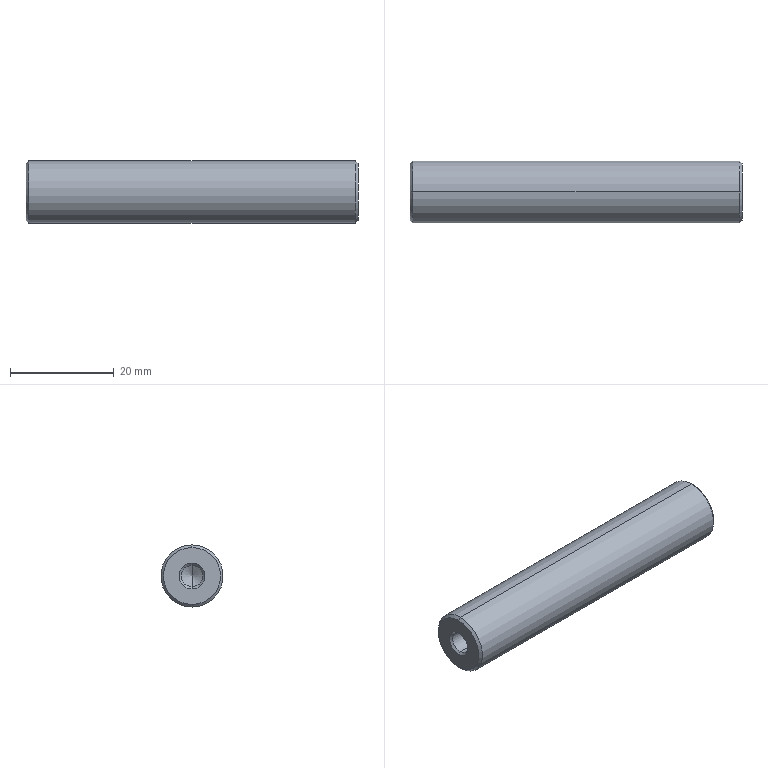Part | STEP file | PSFGT12_64_M5_PSFGT12-64-M5 | 1 solid | 14 faces | box 64 x 12 x 12 mm | volume 7075 mm3 | cone 8 | cylinder 4 | plane 2 | commonest cylinder face diameters 4.134 x2 12 x2
STEP:
#1=CARTESIAN_POINT('',(0.,0.,0.));
#2=DIRECTION('',(0.,0.,1.));
#3=DIRECTION('',(1.,0.,0.));
#4=AXIS2_PLACEMENT_3D('',#1,#2,#3);
#5=CARTESIAN_POINT('',(11.,0.,-2.067));
#6=VERTEX_POINT('',#5);
#7=CARTESIAN_POINT('',(11.,0.,2.067));
#8=VERTEX_POINT('',#7);
#9=CARTESIAN_POINT('',(11.,0.,0.));
#10=DIRECTION('',(-1.,0.,0.));
#11=DIRECTION('',(0.,0.,1.));
#12=AXIS2_PLACEMENT_3D('',#9,#10,#11);
#13=CIRCLE('',#12,2.067);
#14=CARTESIAN_POINT('',(-987.807,0.,0.));
#15=DIRECTION('',(-1.,0.,0.));
#16=DIRECTION('',(0.,0.,1.));
#17=AXIS2_PLACEMENT_3D('',#14,#15,#16);
#18=CONICAL_SURFACE('',#17,1732.051,1.047);
#19=CARTESIAN_POINT('',(0.,-998.807));
#20=DIRECTION('',(1.,0.));
#21=VECTOR('',#20,1.);
#22=LINE('',#19,#21);
#23=(GEOMETRIC_REPRESENTATION_CONTEXT(2)PARAMETRIC_REPRESENTATION_CONTEXT()REPRESENTATION_CONTEXT('',''));
#24=DEFINITIONAL_REPRESENTATION('',(#22),#23);
#25=PCURVE('',#18,#24);
#26=CARTESIAN_POINT('',(12.193,0.,0.));
#27=DIRECTION('',(-1.,0.,0.));
#28=DIRECTION('',(0.,0.,1.));
#29=AXIS2_PLACEMENT_3D('',#26,#27,#28);
#30=CYLINDRICAL_SURFACE('',#29,2.067);
#31=CARTESIAN_POINT('',(0.,1.193));
#32=DIRECTION('',(1.,0.));
#33=VECTOR('',#32,1.);
#34=LINE('',#31,#33);
#35=(GEOMETRIC_REPRESENTATION_CONTEXT(2)PARAMETRIC_REPRESENTATION_CONTEXT()REPRESENTATION_CONTEXT('',''));
#36=DEFINITIONAL_REPRESENTATION('',(#34),#35);
#37=PCURVE('',#30,#36);
#38=SURFACE_CURVE('',#13,(#25,#37),.PCURVE_S1.);
#39=EDGE_CURVE('',#6,#8,#38,.T.);
#40=ORIENTED_EDGE('',*,*,#39,.F.);
#41=CARTESIAN_POINT('',(12.193,0.,0.));
#42=VERTEX_POINT('',#41);
#43=CARTESIAN_POINT('',(12.193,0.,0.));
#44=DIRECTION('',(-0.5,0.,-0.866));
#45=VECTOR('',#44,1.);
#46=LINE('',#43,#45);
#47=CARTESIAN_POINT('',(3.142,-1000.));
#48=CARTESIAN_POINT('',(3.142,-999.982));
#49=CARTESIAN_POINT('',(3.142,-999.946));
#50=CARTESIAN_POINT('',(3.142,-999.892));
#51=CARTESIAN_POINT('',(3.142,-999.837));
#52=CARTESIAN_POINT('',(3.142,-999.783));
#53=CARTESIAN_POINT('',(3.142,-999.729));
#54=CARTESIAN_POINT('',(3.142,-999.675));
#55=CARTESIAN_POINT('',(3.142,-999.62));
#56=CARTESIAN_POINT('',(3.142,-999.566));
#57=CARTESIAN_POINT('',(3.142,-999.512));
#58=CARTESIAN_POINT('',(3.142,-999.458));
#59=CARTESIAN_POINT('',(3.142,-999.403));
#60=CARTESIAN_POINT('',(3.142,-999.349));
#61=CARTESIAN_POINT('',(3.142,-999.295));
#62=CARTESIAN_POINT('',(3.142,-999.241));
#63=CARTESIAN_POINT('',(3.142,-999.186));
#64=CARTESIAN_POINT('',(3.142,-999.132));
#65=CARTESIAN_POINT('',(3.142,-999.078));
#66=CARTESIAN_POINT('',(3.142,-999.024));
#67=CARTESIAN_POINT('',(3.142,-998.969));
#68=CARTESIAN_POINT('',(3.142,-998.915));
#69=CARTESIAN_POINT('',(3.142,-998.861));
#70=CARTESIAN_POINT('',(3.142,-998.825));
#71=CARTESIAN_POINT('',(3.142,-998.807));
#72=B_SPLINE_CURVE_WITH_KNOTS('',3,(#47,#48,#49,#50,#51,#52,#53,#54,#55,#56,#57,#58,#59,#60,#61,#62,#63,#64,#65,#66,#67,#68,#69,#70,#71),.UNSPECIFIED.,.F.,.F.,(4,1,1,1,1,1,1,1,1,1,1,1,1,1,1,1,1,1,1,1,1,1,4),(0.,0.1085,0.217,0.3255,0.434,0.5424,0.6509,0.7594,0.8679,0.9764,1.085,1.193,1.302,1.41,1.519,1.627,1.736,1.844,1.953,2.061,2.17,2.278,2.387),.QUASI_UNIFORM_KNOTS.);
#73=(GEOMETRIC_REPRESENTATION_CONTEXT(2)PARAMETRIC_REPRESENTATION_CONTEXT()REPRESENTATION_CONTEXT('',''));
#74=DEFINITIONAL_REPRESENTATION('',(#72),#73);
#75=PCURVE('',#18,#74);
#76=CARTESIAN_POINT('',(-987.807,0.,0.));
#77=DIRECTION('',(-1.,0.,0.));
#78=DIRECTION('',(0.,0.,1.));
#79=AXIS2_PLACEMENT_3D('',#76,#77,#78);
#80=CONICAL_SURFACE('',#79,1732.051,1.047);
#81=CARTESIAN_POINT('',(3.142,-1000.));
#82=CARTESIAN_POINT('',(3.142,-999.982));
#83=CARTESIAN_POINT('',(3.142,-999.946));
#84=CARTESIAN_POINT('',(3.142,-999.892));
#85=CARTESIAN_POINT('',(3.142,-999.837));
#86=CARTESIAN_POINT('',(3.142,-999.783));
#87=CARTESIAN_POINT('',(3.142,-999.729));
#88=CARTESIAN_POINT('',(3.142,-999.675));
#89=CARTESIAN_POINT('',(3.142,-999.62));
#90=CARTESIAN_POINT('',(3.142,-999.566));
#91=CARTESIAN_POINT('',(3.142,-999.512));
#92=CARTESIAN_POINT('',(3.142,-999.458));
#93=CARTESIAN_POINT('',(3.142,-999.403));
#94=CARTESIAN_POINT('',(3.142,-999.349));
#95=CARTESIAN_POINT('',(3.142,-999.295));
#96=CARTESIAN_POINT('',(3.142,-999.241));
#97=CARTESIAN_POINT('',(3.142,-999.186));
#98=CARTESIAN_POINT('',(3.142,-999.132));
#99=CARTESIAN_POINT('',(3.142,-999.078));
#100=CARTESIAN_POINT('',(3.142,-999.024));
#101=CARTESIAN_POINT('',(3.142,-998.969));
#102=CARTESIAN_POINT('',(3.142,-998.915));
#103=CARTESIAN_POINT('',(3.142,-998.861));
#104=CARTESIAN_POINT('',(3.142,-998.825));
#105=CARTESIAN_POINT('',(3.142,-998.807));
#106=B_SPLINE_CURVE_WITH_KNOTS('',3,(#81,#82,#83,#84,#85,#86,#87,#88,#89,#90,#91,#92,#93,#94,#95,#96,#97,#98,#99,#100,#101,#102,#103,#104,#105),.UNSPECIFIED.,.F.,.F.,(4,1,1,1,1,1,1,1,1,1,1,1,1,1,1,1,1,1,1,1,1,1,4),(0.,0.1085,0.217,0.3255,0.434,0.5424,0.6509,0.7594,0.8679,0.9764,1.085,1.193,1.302,1.41,1.519,1.627,1.736,1.844,1.953,2.061,2.17,2.278,2.387),.QUASI_UNIFORM_KNOTS.);
#107=(GEOMETRIC_REPRESENTATION_CONTEXT(2)PARAMETRIC_REPRESENTATION_CONTEXT()REPRESENTATION_CONTEXT('',''));
#108=DEFINITIONAL_REPRESENTATION('',(#106),#107);
#109=PCURVE('',#80,#108);
#110=SURFACE_CURVE('',#46,(#75,#109),.PCURVE_S1.);
#111=EDGE_CURVE('',#42,#6,#110,.T.);
#112=ORIENTED_EDGE('',*,*,#111,.F.);
#113=CARTESIAN_POINT('',(12.193,0.,0.));
#114=DIRECTION('',(-0.5,0.,0.866));
#115=VECTOR('',#114,1.);
#116=LINE('',#113,#115);
#117=CARTESIAN_POINT('',(6.283,-1000.));
#118=DIRECTION('',(0.,1.));
#119=VECTOR('',#118,1.);
#120=LINE('',#117,#119);
#121=(GEOMETRIC_REPRESENTATION_CONTEXT(2)PARAMETRIC_REPRESENTATION_CONTEXT()REPRESENTATION_CONTEXT('',''));
#122=DEFINITIONAL_REPRESENTATION('',(#120),#121);
#123=PCURVE('',#18,#122);
#124=CARTESIAN_POINT('',(0.,-1000.));
#125=DIRECTION('',(0.,1.));
#126=VECTOR('',#125,1.);
#127=LINE('',#124,#126);
#128=(GEOMETRIC_REPRESENTATION_CONTEXT(2)PARAMETRIC_REPRESENTATION_CONTEXT()REPRESENTATION_CONTEXT('',''));
#129=DEFINITIONAL_REPRESENTATION('',(#127),#128);
#130=PCURVE('',#80,#129);
#131=SURFACE_CURVE('',#116,(#123,#130),.PCURVE_S1.);
#132=EDGE_CURVE('',#42,#8,#131,.T.);
#133=ORIENTED_EDGE('',*,*,#132,.T.);
#134=EDGE_LOOP('',(#40,#112,#133));
#135=FACE_BOUND('',#134,.F.);
#136=ADVANCED_FACE('',(#135),#18,.F.);
#137=CARTESIAN_POINT('',(0.433,0.,2.067));
#138=VERTEX_POINT('',#137);
#139=CARTESIAN_POINT('',(12.193,0.,2.067));
#140=DIRECTION('',(-1.,0.,0.));
#141=VECTOR('',#140,1.);
#142=LINE('',#139,#141);
#143=CARTESIAN_POINT('',(6.283,0.));
#144=DIRECTION('',(0.,1.));
#145=VECTOR('',#144,1.);
#146=LINE('',#143,#145);
#147=(GEOMETRIC_REPRESENTATION_CONTEXT(2)PARAMETRIC_REPRESENTATION_CONTEXT()REPRESENTATION_CONTEXT('',''));
#148=DEFINITIONAL_REPRESENTATION('',(#146),#147);
#149=PCURVE('',#30,#148);
#150=CARTESIAN_POINT('',(12.193,0.,0.));
#151=DIRECTION('',(-1.,0.,0.));
#152=DIRECTION('',(0.,0.,1.));
#153=AXIS2_PLACEMENT_3D('',#150,#151,#152);
#154=CYLINDRICAL_SURFACE('',#153,2.067);
#155=CARTESIAN_POINT('',(0.,0.));
#156=DIRECTION('',(0.,1.));
#157=VECTOR('',#156,1.);
#158=LINE('',#155,#157);
#159=(GEOMETRIC_REPRESENTATION_CONTEXT(2)PARAMETRIC_REPRESENTATION_CONTEXT()REPRESENTATION_CONTEXT('',''));
#160=DEFINITIONAL_REPRESENTATION('',(#158),#159);
#161=PCURVE('',#154,#160);
#162=SURFACE_CURVE('',#142,(#149,#161),.PCURVE_S1.);
#163=EDGE_CURVE('',#8,#138,#162,.T.);
#164=ORIENTED_EDGE('',*,*,#163,.T.);
#165=CARTESIAN_POINT('',(0.433,0.,-2.067));
#166=VERTEX_POINT('',#165);
#167=CARTESIAN_POINT('',(0.433,0.,0.));
#168=DIRECTION('',(-1.,0.,0.));
#169=DIRECTION('',(0.,0.,1.));
#170=AXIS2_PLACEMENT_3D('',#167,#168,#169);
#171=CIRCLE('',#170,2.067);
#172=CARTESIAN_POINT('',(0.,11.76));
#173=DIRECTION('',(1.,0.));
#174=VECTOR('',#173,1.);
#175=LINE('',#172,#174);
#176=(GEOMETRIC_REPRESENTATION_CONTEXT(2)PARAMETRIC_REPRESENTATION_CONTEXT()REPRESENTATION_CONTEXT('',''));
#177=DEFINITIONAL_REPRESENTATION('',(#175),#176);
#178=PCURVE('',#30,#177);
#179=CARTESIAN_POINT('',(0.433,0.,0.));
#180=DIRECTION('',(-1.,0.,0.));
#181=DIRECTION('',(0.,0.,1.));
#182=AXIS2_PLACEMENT_3D('',#179,#180,#181);
#183=CONICAL_SURFACE('',#182,2.067,0.7854);
#184=CARTESIAN_POINT('',(0.,0.));
#185=DIRECTION('',(1.,0.));
#186=VECTOR('',#185,1.);
#187=LINE('',#184,#186);
#188=(GEOMETRIC_REPRESENTATION_CONTEXT(2)PARAMETRIC_REPRESENTATION_CONTEXT()REPRESENTATION_CONTEXT('',''));
#189=DEFINITIONAL_REPRESENTATION('',(#187),#188);
#190=PCURVE('',#183,#189);
#191=SURFACE_CURVE('',#171,(#178,#190),.PCURVE_S1.);
#192=EDGE_CURVE('',#166,#138,#191,.T.);
#193=ORIENTED_EDGE('',*,*,#192,.F.);
#194=CARTESIAN_POINT('',(12.193,0.,-2.067));
#195=DIRECTION('',(-1.,0.,0.));
#196=VECTOR('',#195,1.);
#197=LINE('',#194,#196);
#198=CARTESIAN_POINT('',(3.142,0.));
#199=DIRECTION('',(0.,1.));
#200=VECTOR('',#199,1.);
#201=LINE('',#198,#200);
#202=(GEOMETRIC_REPRESENTATION_CONTEXT(2)PARAMETRIC_REPRESENTATION_CONTEXT()REPRESENTATION_CONTEXT('',''));
#203=DEFINITIONAL_REPRESENTATION('',(#201),#202);
#204=PCURVE('',#30,#203);
#205=CARTESIAN_POINT('',(3.142,0.));
#206=DIRECTION('',(0.,1.));
#207=VECTOR('',#206,1.);
#208=LINE('',#205,#207);
#209=(GEOMETRIC_REPRESENTATION_CONTEXT(2)PARAMETRIC_REPRESENTATION_CONTEXT()REPRESENTATION_CONTEXT('',''));
#210=DEFINITIONAL_REPRESENTATION('',(#208),#209);
#211=PCURVE('',#154,#210);
#212=SURFACE_CURVE('',#197,(#204,#211),.PCURVE_S1.);
#213=EDGE_CURVE('',#6,#166,#212,.T.);
#214=ORIENTED_EDGE('',*,*,#213,.F.);
#215=ORIENTED_EDGE('',*,*,#39,.T.);
#216=EDGE_LOOP('',(#164,#193,#214,#215));
#217=FACE_BOUND('',#216,.F.);
#218=ADVANCED_FACE('',(#217),#30,.F.);
#219=CARTESIAN_POINT('',(0.,0.,2.5));
#220=VERTEX_POINT('',#219);
#221=CARTESIAN_POINT('',(0.433,0.,2.067));
#222=DIRECTION('',(-0.7071,0.,0.7071));
#223=VECTOR('',#222,1.);
#224=LINE('',#221,#223);
#225=CARTESIAN_POINT('',(6.283,0.));
#226=DIRECTION('',(0.,1.));
#227=VECTOR('',#226,1.);
#228=LINE('',#225,#227);
#229=(GEOMETRIC_REPRESENTATION_CONTEXT(2)PARAMETRIC_REPRESENTATION_CONTEXT()REPRESENTATION_CONTEXT('',''));
#230=DEFINITIONAL_REPRESENTATION('',(#228),#229);
#231=PCURVE('',#183,#230);
#232=CARTESIAN_POINT('',(0.433,0.,0.));
#233=DIRECTION('',(-1.,0.,0.));
#234=DIRECTION('',(0.,0.,1.));
#235=AXIS2_PLACEMENT_3D('',#232,#233,#234);
#236=CONICAL_SURFACE('',#235,2.067,0.7854);
#237=CARTESIAN_POINT('',(0.,0.));
#238=DIRECTION('',(0.,1.));
#239=VECTOR('',#238,1.);
#240=LINE('',#237,#239);
#241=(GEOMETRIC_REPRESENTATION_CONTEXT(2)PARAMETRIC_REPRESENTATION_CONTEXT()REPRESENTATION_CONTEXT('',''));
#242=DEFINITIONAL_REPRESENTATION('',(#240),#241);
#243=PCURVE('',#236,#242);
#244=SURFACE_CURVE('',#224,(#231,#243),.PCURVE_S1.);
#245=EDGE_CURVE('',#138,#220,#244,.T.);
#246=ORIENTED_EDGE('',*,*,#245,.T.);
#247=CARTESIAN_POINT('',(0.,0.,-2.5));
#248=VERTEX_POINT('',#247);
#249=CARTESIAN_POINT('',(0.,0.,0.));
#250=DIRECTION('',(-1.,0.,0.));
#251=DIRECTION('',(0.,0.,1.));
#252=AXIS2_PLACEMENT_3D('',#249,#250,#251);
#253=CIRCLE('',#252,2.5);
#254=CARTESIAN_POINT('',(0.,0.433));
#255=DIRECTION('',(1.,0.));
#256=VECTOR('',#255,1.);
#257=LINE('',#254,#256);
#258=(GEOMETRIC_REPRESENTATION_CONTEXT(2)PARAMETRIC_REPRESENTATION_CONTEXT()REPRESENTATION_CONTEXT('',''));
#259=DEFINITIONAL_REPRESENTATION('',(#257),#258);
#260=PCURVE('',#183,#259);
#261=CARTESIAN_POINT('',(0.,0.,0.));
#262=DIRECTION('',(1.,0.,0.));
#263=DIRECTION('',(0.,0.,-1.));
#264=AXIS2_PLACEMENT_3D('',#261,#262,#263);
#265=PLANE('',#264);
#266=CARTESIAN_POINT('',(-2.5,0.));
#267=CARTESIAN_POINT('',(-2.5,4.33));
#268=CARTESIAN_POINT('',(1.25,2.165));
#269=CARTESIAN_POINT('',(5.,0.));
#270=CARTESIAN_POINT('',(1.25,-2.165));
#271=CARTESIAN_POINT('',(-2.5,-4.33));
#272=CARTESIAN_POINT('',(-2.5,0.));
#273=(BOUNDED_CURVE()B_SPLINE_CURVE(2,(#266,#267,#268,#269,#270,#271,#272),.UNSPECIFIED.,.T.,.F.)B_SPLINE_CURVE_WITH_KNOTS((1,2,2,2,2,1),(-2.094,0.,2.094,4.189,6.283,8.378),.UNSPECIFIED.)CURVE()GEOMETRIC_REPRESENTATION_ITEM()RATIONAL_B_SPLINE_CURVE((1.,0.5,1.,0.5,1.,0.5,1.))REPRESENTATION_ITEM(''));
#274=(GEOMETRIC_REPRESENTATION_CONTEXT(2)PARAMETRIC_REPRESENTATION_CONTEXT()REPRESENTATION_CONTEXT('',''));
#275=DEFINITIONAL_REPRESENTATION('',(#273),#274);
#276=PCURVE('',#265,#275);
#277=SURFACE_CURVE('',#253,(#260,#276),.PCURVE_S1.);
#278=EDGE_CURVE('',#248,#220,#277,.T.);
#279=ORIENTED_EDGE('',*,*,#278,.F.);
#280=CARTESIAN_POINT('',(0.433,0.,-2.067));
#281=DIRECTION('',(-0.7071,0.,-0.7071));
#282=VECTOR('',#281,1.);
#283=LINE('',#280,#282);
#284=CARTESIAN_POINT('',(3.142,0.));
#285=DIRECTION('',(0.,1.));
#286=VECTOR('',#285,1.);
#287=LINE('',#284,#286);
#288=(GEOMETRIC_REPRESENTATION_CONTEXT(2)PARAMETRIC_REPRESENTATION_CONTEXT()REPRESENTATION_CONTEXT('',''));
#289=DEFINITIONAL_REPRESENTATION('',(#287),#288);
#290=PCURVE('',#183,#289);
#291=CARTESIAN_POINT('',(3.142,0.));
#292=DIRECTION('',(0.,1.));
#293=VECTOR('',#292,1.);
#294=LINE('',#291,#293);
#295=(GEOMETRIC_REPRESENTATION_CONTEXT(2)PARAMETRIC_REPRESENTATION_CONTEXT()REPRESENTATION_CONTEXT('',''));
#296=DEFINITIONAL_REPRESENTATION('',(#294),#295);
#297=PCURVE('',#236,#296);
#298=SURFACE_CURVE('',#283,(#290,#297),.PCURVE_S1.);
#299=EDGE_CURVE('',#166,#248,#298,.T.);
#300=ORIENTED_EDGE('',*,*,#299,.F.);
#301=ORIENTED_EDGE('',*,*,#192,.T.);
#302=EDGE_LOOP('',(#246,#279,#300,#301));
#303=FACE_BOUND('',#302,.F.);
#304=ADVANCED_FACE('',(#303),#183,.F.);
#305=CARTESIAN_POINT('',(64.,0.,5.5));
#306=VERTEX_POINT('',#305);
#307=CARTESIAN_POINT('',(64.,0.,-5.5));
#308=VERTEX_POINT('',#307);
#309=CARTESIAN_POINT('',(64.,0.,0.));
#310=DIRECTION('',(-1.,0.,0.));
#311=DIRECTION('',(0.,0.,1.));
#312=AXIS2_PLACEMENT_3D('',#309,#310,#311);
#313=CIRCLE('',#312,5.5);
#314=CARTESIAN_POINT('',(64.,0.,0.));
#315=DIRECTION('',(-1.,0.,0.));
#316=DIRECTION('',(0.,0.,1.));
#317=AXIS2_PLACEMENT_3D('',#314,#315,#316);
#318=CONICAL_SURFACE('',#317,5.5,0.7854);
#319=CARTESIAN_POINT('',(0.,0.));
#320=DIRECTION('',(1.,0.));
#321=VECTOR('',#320,1.);
#322=LINE('',#319,#321);
#323=(GEOMETRIC_REPRESENTATION_CONTEXT(2)PARAMETRIC_REPRESENTATION_CONTEXT()REPRESENTATION_CONTEXT('',''));
#324=DEFINITIONAL_REPRESENTATION('',(#322),#323);
#325=PCURVE('',#318,#324);
#326=CARTESIAN_POINT('',(64.,5.5,0.));
#327=DIRECTION('',(-1.,0.,0.));
#328=DIRECTION('',(0.,0.,1.));
#329=AXIS2_PLACEMENT_3D('',#326,#327,#328);
#330=PLANE('',#329);
#331=CARTESIAN_POINT('',(0.,-5.5));
#332=DIRECTION('',(1.,0.));
#333=AXIS2_PLACEMENT_2D('',#331,#332);
#334=CIRCLE('',#333,5.5);
#335=(GEOMETRIC_REPRESENTATION_CONTEXT(2)PARAMETRIC_REPRESENTATION_CONTEXT()REPRESENTATION_CONTEXT('',''));
#336=DEFINITIONAL_REPRESENTATION('',(#334),#335);
#337=PCURVE('',#330,#336);
#338=SURFACE_CURVE('',#313,(#325,#337),.PCURVE_S1.);
#339=EDGE_CURVE('',#306,#308,#338,.T.);
#340=ORIENTED_EDGE('',*,*,#339,.T.);
#341=CARTESIAN_POINT('',(63.5,0.,-6.));
#342=VERTEX_POINT('',#341);
#343=CARTESIAN_POINT('',(64.,0.,-5.5));
#344=DIRECTION('',(-0.7071,0.,-0.7071));
#345=VECTOR('',#344,1.);
#346=LINE('',#343,#345);
#347=CARTESIAN_POINT('',(3.142,0.));
#348=DIRECTION('',(0.,1.));
#349=VECTOR('',#348,1.);
#350=LINE('',#347,#349);
#351=(GEOMETRIC_REPRESENTATION_CONTEXT(2)PARAMETRIC_REPRESENTATION_CONTEXT()REPRESENTATION_CONTEXT('',''));
#352=DEFINITIONAL_REPRESENTATION('',(#350),#351);
#353=PCURVE('',#318,#352);
#354=CARTESIAN_POINT('',(64.,0.,0.));
#355=DIRECTION('',(-1.,0.,0.));
#356=DIRECTION('',(0.,0.,1.));
#357=AXIS2_PLACEMENT_3D('',#354,#355,#356);
#358=CONICAL_SURFACE('',#357,5.5,0.7854);
#359=CARTESIAN_POINT('',(3.142,0.));
#360=DIRECTION('',(0.,1.));
#361=VECTOR('',#360,1.);
#362=LINE('',#359,#361);
#363=(GEOMETRIC_REPRESENTATION_CONTEXT(2)PARAMETRIC_REPRESENTATION_CONTEXT()REPRESENTATION_CONTEXT('',''));
#364=DEFINITIONAL_REPRESENTATION('',(#362),#363);
#365=PCURVE('',#358,#364);
#366=SURFACE_CURVE('',#346,(#353,#365),.PCURVE_S1.);
#367=EDGE_CURVE('',#308,#342,#366,.T.);
#368=ORIENTED_EDGE('',*,*,#367,.T.);
#369=CARTESIAN_POINT('',(63.5,0.,6.));
#370=VERTEX_POINT('',#369);
#371=CARTESIAN_POINT('',(63.5,0.,0.));
#372=DIRECTION('',(-1.,0.,0.));
#373=DIRECTION('',(0.,0.,1.));
#374=AXIS2_PLACEMENT_3D('',#371,#372,#373);
#375=CIRCLE('',#374,6.);
#376=CARTESIAN_POINT('',(0.,0.5));
#377=DIRECTION('',(1.,0.));
#378=VECTOR('',#377,1.);
#379=LINE('',#376,#378);
#380=(GEOMETRIC_REPRESENTATION_CONTEXT(2)PARAMETRIC_REPRESENTATION_CONTEXT()REPRESENTATION_CONTEXT('',''));
#381=DEFINITIONAL_REPRESENTATION('',(#379),#380);
#382=PCURVE('',#318,#381);
#383=CARTESIAN_POINT('',(64.,0.,0.));
#384=DIRECTION('',(-1.,0.,0.));
#385=DIRECTION('',(0.,0.,1.));
#386=AXIS2_PLACEMENT_3D('',#383,#384,#385);
#387=CYLINDRICAL_SURFACE('',#386,6.);
#388=CARTESIAN_POINT('',(0.,0.5));
#389=DIRECTION('',(1.,0.));
#390=VECTOR('',#389,1.);
#391=LINE('',#388,#390);
#392=(GEOMETRIC_REPRESENTATION_CONTEXT(2)PARAMETRIC_REPRESENTATION_CONTEXT()REPRESENTATION_CONTEXT('',''));
#393=DEFINITIONAL_REPRESENTATION('',(#391),#392);
#394=PCURVE('',#387,#393);
#395=SURFACE_CURVE('',#375,(#382,#394),.PCURVE_S1.);
#396=EDGE_CURVE('',#370,#342,#395,.T.);
#397=ORIENTED_EDGE('',*,*,#396,.F.);
#398=CARTESIAN_POINT('',(64.,0.,5.5));
#399=DIRECTION('',(-0.7071,0.,0.7071));
#400=VECTOR('',#399,1.);
#401=LINE('',#398,#400);
#402=CARTESIAN_POINT('',(0.,0.));
#403=DIRECTION('',(0.,1.));
#404=VECTOR('',#403,1.);
#405=LINE('',#402,#404);
#406=(GEOMETRIC_REPRESENTATION_CONTEXT(2)PARAMETRIC_REPRESENTATION_CONTEXT()REPRESENTATION_CONTEXT('',''));
#407=DEFINITIONAL_REPRESENTATION('',(#405),#406);
#408=PCURVE('',#318,#407);
#409=CARTESIAN_POINT('',(6.283,0.));
#410=DIRECTION('',(0.,1.));
#411=VECTOR('',#410,1.);
#412=LINE('',#409,#411);
#413=(GEOMETRIC_REPRESENTATION_CONTEXT(2)PARAMETRIC_REPRESENTATION_CONTEXT()REPRESENTATION_CONTEXT('',''));
#414=DEFINITIONAL_REPRESENTATION('',(#412),#413);
#415=PCURVE('',#358,#414);
#416=SURFACE_CURVE('',#401,(#408,#415),.PCURVE_S1.);
#417=EDGE_CURVE('',#306,#370,#416,.T.);
#418=ORIENTED_EDGE('',*,*,#417,.F.);
#419=EDGE_LOOP('',(#340,#368,#397,#418));
#420=FACE_BOUND('',#419,.T.);
#421=ADVANCED_FACE('',(#420),#318,.T.);
#422=ORIENTED_EDGE('',*,*,#396,.T.);
#423=CARTESIAN_POINT('',(0.5,0.,-6.));
#424=VERTEX_POINT('',#423);
#425=CARTESIAN_POINT('',(64.,0.,-6.));
#426=DIRECTION('',(-1.,0.,0.));
#427=VECTOR('',#426,1.);
#428=LINE('',#425,#427);
#429=CARTESIAN_POINT('',(3.142,0.));
#430=DIRECTION('',(0.,1.));
#431=VECTOR('',#430,1.);
#432=LINE('',#429,#431);
#433=(GEOMETRIC_REPRESENTATION_CONTEXT(2)PARAMETRIC_REPRESENTATION_CONTEXT()REPRESENTATION_CONTEXT('',''));
#434=DEFINITIONAL_REPRESENTATION('',(#432),#433);
#435=PCURVE('',#387,#434);
#436=CARTESIAN_POINT('',(64.,0.,0.));
#437=DIRECTION('',(-1.,0.,0.));
#438=DIRECTION('',(0.,0.,1.));
#439=AXIS2_PLACEMENT_3D('',#436,#437,#438);
#440=CYLINDRICAL_SURFACE('',#439,6.);
#441=CARTESIAN_POINT('',(3.142,0.));
#442=DIRECTION('',(0.,1.));
#443=VECTOR('',#442,1.);
#444=LINE('',#441,#443);
#445=(GEOMETRIC_REPRESENTATION_CONTEXT(2)PARAMETRIC_REPRESENTATION_CONTEXT()REPRESENTATION_CONTEXT('',''));
#446=DEFINITIONAL_REPRESENTATION('',(#444),#445);
#447=PCURVE('',#440,#446);
#448=SURFACE_CURVE('',#428,(#435,#447),.PCURVE_S1.);
#449=EDGE_CURVE('',#342,#424,#448,.T.);
#450=ORIENTED_EDGE('',*,*,#449,.T.);
#451=CARTESIAN_POINT('',(0.5,0.,6.));
#452=VERTEX_POINT('',#451);
#453=CARTESIAN_POINT('',(0.5,0.,0.));
#454=DIRECTION('',(-1.,0.,0.));
#455=DIRECTION('',(0.,0.,1.));
#456=AXIS2_PLACEMENT_3D('',#453,#454,#455);
#457=CIRCLE('',#456,6.);
#458=CARTESIAN_POINT('',(0.,63.5));
#459=DIRECTION('',(1.,0.));
#460=VECTOR('',#459,1.);
#461=LINE('',#458,#460);
#462=(GEOMETRIC_REPRESENTATION_CONTEXT(2)PARAMETRIC_REPRESENTATION_CONTEXT()REPRESENTATION_CONTEXT('',''));
#463=DEFINITIONAL_REPRESENTATION('',(#461),#462);
#464=PCURVE('',#387,#463);
#465=CARTESIAN_POINT('',(0.5,0.,0.));
#466=DIRECTION('',(1.,0.,0.));
#467=DIRECTION('',(0.,0.,-1.));
#468=AXIS2_PLACEMENT_3D('',#465,#466,#467);
#469=CONICAL_SURFACE('',#468,6.,0.7854);
#470=CARTESIAN_POINT('',(3.142,0.));
#471=DIRECTION('',(-1.,0.));
#472=VECTOR('',#471,1.);
#473=LINE('',#470,#472);
#474=(GEOMETRIC_REPRESENTATION_CONTEXT(2)PARAMETRIC_REPRESENTATION_CONTEXT()REPRESENTATION_CONTEXT('',''));
#475=DEFINITIONAL_REPRESENTATION('',(#473),#474);
#476=PCURVE('',#469,#475);
#477=SURFACE_CURVE('',#457,(#464,#476),.PCURVE_S1.);
#478=EDGE_CURVE('',#452,#424,#477,.T.);
#479=ORIENTED_EDGE('',*,*,#478,.F.);
#480=CARTESIAN_POINT('',(64.,0.,6.));
#481=DIRECTION('',(-1.,0.,0.));
#482=VECTOR('',#481,1.);
#483=LINE('',#480,#482);
#484=CARTESIAN_POINT('',(0.,0.));
#485=DIRECTION('',(0.,1.));
#486=VECTOR('',#485,1.);
#487=LINE('',#484,#486);
#488=(GEOMETRIC_REPRESENTATION_CONTEXT(2)PARAMETRIC_REPRESENTATION_CONTEXT()REPRESENTATION_CONTEXT('',''));
#489=DEFINITIONAL_REPRESENTATION('',(#487),#488);
#490=PCURVE('',#387,#489);
#491=CARTESIAN_POINT('',(6.283,0.));
#492=DIRECTION('',(0.,1.));
#493=VECTOR('',#492,1.);
#494=LINE('',#491,#493);
#495=(GEOMETRIC_REPRESENTATION_CONTEXT(2)PARAMETRIC_REPRESENTATION_CONTEXT()REPRESENTATION_CONTEXT('',''));
#496=DEFINITIONAL_REPRESENTATION('',(#494),#495);
#497=PCURVE('',#440,#496);
#498=SURFACE_CURVE('',#483,(#490,#497),.PCURVE_S1.);
#499=EDGE_CURVE('',#370,#452,#498,.T.);
#500=ORIENTED_EDGE('',*,*,#499,.F.);
#501=EDGE_LOOP('',(#422,#450,#479,#500));
#502=FACE_BOUND('',#501,.T.);
#503=ADVANCED_FACE('',(#502),#387,.T.);
#504=CARTESIAN_POINT('',(0.,0.,5.5));
#505=VERTEX_POINT('',#504);
#506=CARTESIAN_POINT('',(0.,0.,-5.5));
#507=VERTEX_POINT('',#506);
#508=CARTESIAN_POINT('',(0.,0.,0.));
#509=DIRECTION('',(-1.,0.,0.));
#510=DIRECTION('',(0.,0.,1.));
#511=AXIS2_PLACEMENT_3D('',#508,#509,#510);
#512=CIRCLE('',#511,5.5);
#513=CARTESIAN_POINT('',(3.142,-0.5));
#514=DIRECTION('',(-1.,0.));
#515=VECTOR('',#514,1.);
#516=LINE('',#513,#515);
#517=(GEOMETRIC_REPRESENTATION_CONTEXT(2)PARAMETRIC_REPRESENTATION_CONTEXT()REPRESENTATION_CONTEXT('',''));
#518=DEFINITIONAL_REPRESENTATION('',(#516),#517);
#519=PCURVE('',#469,#518);
#520=CARTESIAN_POINT('',(-5.5,0.));
#521=CARTESIAN_POINT('',(-5.5,9.526));
#522=CARTESIAN_POINT('',(2.75,4.763));
#523=CARTESIAN_POINT('',(11.,0.));
#524=CARTESIAN_POINT('',(2.75,-4.763));
#525=CARTESIAN_POINT('',(-5.5,-9.526));
#526=CARTESIAN_POINT('',(-5.5,0.));
#527=(BOUNDED_CURVE()B_SPLINE_CURVE(2,(#520,#521,#522,#523,#524,#525,#526),.UNSPECIFIED.,.T.,.F.)B_SPLINE_CURVE_WITH_KNOTS((1,2,2,2,2,1),(-2.094,0.,2.094,4.189,6.283,8.378),.UNSPECIFIED.)CURVE()GEOMETRIC_REPRESENTATION_ITEM()RATIONAL_B_SPLINE_CURVE((1.,0.5,1.,0.5,1.,0.5,1.))REPRESENTATION_ITEM(''));
#528=(GEOMETRIC_REPRESENTATION_CONTEXT(2)PARAMETRIC_REPRESENTATION_CONTEXT()REPRESENTATION_CONTEXT('',''));
#529=DEFINITIONAL_REPRESENTATION('',(#527),#528);
#530=PCURVE('',#265,#529);
#531=SURFACE_CURVE('',#512,(#519,#530),.PCURVE_S1.);
#532=EDGE_CURVE('',#505,#507,#531,.T.);
#533=ORIENTED_EDGE('',*,*,#532,.F.);
#534=CARTESIAN_POINT('',(0.5,0.,6.));
#535=DIRECTION('',(0.7071,0.,0.7071));
#536=VECTOR('',#535,1.);
#537=LINE('',#534,#536);
#538=CARTESIAN_POINT('',(3.142,0.));
#539=DIRECTION('',(0.,1.));
#540=VECTOR('',#539,1.);
#541=LINE('',#538,#540);
#542=(GEOMETRIC_REPRESENTATION_CONTEXT(2)PARAMETRIC_REPRESENTATION_CONTEXT()REPRESENTATION_CONTEXT('',''));
#543=DEFINITIONAL_REPRESENTATION('',(#541),#542);
#544=PCURVE('',#469,#543);
#545=CARTESIAN_POINT('',(0.5,0.,0.));
#546=DIRECTION('',(1.,0.,0.));
#547=DIRECTION('',(0.,0.,-1.));
#548=AXIS2_PLACEMENT_3D('',#545,#546,#547);
#549=CONICAL_SURFACE('',#548,6.,0.7854);
#550=CARTESIAN_POINT('',(3.142,0.));
#551=DIRECTION('',(0.,1.));
#552=VECTOR('',#551,1.);
#553=LINE('',#550,#552);
#554=(GEOMETRIC_REPRESENTATION_CONTEXT(2)PARAMETRIC_REPRESENTATION_CONTEXT()REPRESENTATION_CONTEXT('',''));
#555=DEFINITIONAL_REPRESENTATION('',(#553),#554);
#556=PCURVE('',#549,#555);
#557=SURFACE_CURVE('',#537,(#544,#556),.PCURVE_S1.);
#558=EDGE_CURVE('',#505,#452,#557,.T.);
#559=ORIENTED_EDGE('',*,*,#558,.T.);
#560=ORIENTED_EDGE('',*,*,#478,.T.);
#561=CARTESIAN_POINT('',(0.5,0.,-6.));
#562=DIRECTION('',(0.7071,0.,-0.7071));
#563=VECTOR('',#562,1.);
#564=LINE('',#561,#563);
#565=CARTESIAN_POINT('',(0.,0.));
#566=DIRECTION('',(0.,1.));
#567=VECTOR('',#566,1.);
#568=LINE('',#565,#567);
#569=(GEOMETRIC_REPRESENTATION_CONTEXT(2)PARAMETRIC_REPRESENTATION_CONTEXT()REPRESENTATION_CONTEXT('',''));
#570=DEFINITIONAL_REPRESENTATION('',(#568),#569);
#571=PCURVE('',#469,#570);
#572=CARTESIAN_POINT('',(6.283,0.));
#573=DIRECTION('',(0.,1.));
#574=VECTOR('',#573,1.);
#575=LINE('',#572,#574);
#576=(GEOMETRIC_REPRESENTATION_CONTEXT(2)PARAMETRIC_REPRESENTATION_CONTEXT()REPRESENTATION_CONTEXT('',''));
#577=DEFINITIONAL_REPRESENTATION('',(#575),#576);
#578=PCURVE('',#549,#577);
#579=SURFACE_CURVE('',#564,(#571,#578),.PCURVE_S1.);
#580=EDGE_CURVE('',#507,#424,#579,.T.);
#581=ORIENTED_EDGE('',*,*,#580,.F.);
#582=EDGE_LOOP('',(#533,#559,#560,#581));
#583=FACE_BOUND('',#582,.T.);
#584=ADVANCED_FACE('',(#583),#469,.T.);
#585=CARTESIAN_POINT('',(0.,0.,0.));
#586=DIRECTION('',(-1.,0.,0.));
#587=DIRECTION('',(0.,0.,1.));
#588=AXIS2_PLACEMENT_3D('',#585,#586,#587);
#589=CIRCLE('',#588,5.5);
#590=CARTESIAN_POINT('',(-5.5,0.));
#591=CARTESIAN_POINT('',(-5.5,9.526));
#592=CARTESIAN_POINT('',(2.75,4.763));
#593=CARTESIAN_POINT('',(11.,0.));
#594=CARTESIAN_POINT('',(2.75,-4.763));
#595=CARTESIAN_POINT('',(-5.5,-9.526));
#596=CARTESIAN_POINT('',(-5.5,0.));
#597=(BOUNDED_CURVE()B_SPLINE_CURVE(2,(#590,#591,#592,#593,#594,#595,#596),.UNSPECIFIED.,.T.,.F.)B_SPLINE_CURVE_WITH_KNOTS((1,2,2,2,2,1),(-2.094,0.,2.094,4.189,6.283,8.378),.UNSPECIFIED.)CURVE()GEOMETRIC_REPRESENTATION_ITEM()RATIONAL_B_SPLINE_CURVE((1.,0.5,1.,0.5,1.,0.5,1.))REPRESENTATION_ITEM(''));
#598=(GEOMETRIC_REPRESENTATION_CONTEXT(2)PARAMETRIC_REPRESENTATION_CONTEXT()REPRESENTATION_CONTEXT('',''));
#599=DEFINITIONAL_REPRESENTATION('',(#597),#598);
#600=PCURVE('',#265,#599);
#601=CARTESIAN_POINT('',(9.425,-0.5));
#602=DIRECTION('',(-1.,0.));
#603=VECTOR('',#602,1.);
#604=LINE('',#601,#603);
#605=(GEOMETRIC_REPRESENTATION_CONTEXT(2)PARAMETRIC_REPRESENTATION_CONTEXT()REPRESENTATION_CONTEXT('',''));
#606=DEFINITIONAL_REPRESENTATION('',(#604),#605);
#607=PCURVE('',#549,#606);
#608=SURFACE_CURVE('',#589,(#600,#607),.PCURVE_S1.);
#609=EDGE_CURVE('',#507,#505,#608,.T.);
#610=ORIENTED_EDGE('',*,*,#609,.T.);
#611=ORIENTED_EDGE('',*,*,#532,.T.);
#612=EDGE_LOOP('',(#610,#611));
#613=FACE_BOUND('',#612,.T.);
#614=CARTESIAN_POINT('',(0.,0.,0.));
#615=DIRECTION('',(-1.,0.,0.));
#616=DIRECTION('',(0.,0.,1.));
#617=AXIS2_PLACEMENT_3D('',#614,#615,#616);
#618=CIRCLE('',#617,2.5);
#619=CARTESIAN_POINT('',(-2.5,0.));
#620=CARTESIAN_POINT('',(-2.5,4.33));
#621=CARTESIAN_POINT('',(1.25,2.165));
#622=CARTESIAN_POINT('',(5.,0.));
#623=CARTESIAN_POINT('',(1.25,-2.165));
#624=CARTESIAN_POINT('',(-2.5,-4.33));
#625=CARTESIAN_POINT('',(-2.5,0.));
#626=(BOUNDED_CURVE()B_SPLINE_CURVE(2,(#619,#620,#621,#622,#623,#624,#625),.UNSPECIFIED.,.T.,.F.)B_SPLINE_CURVE_WITH_KNOTS((1,2,2,2,2,1),(-2.094,0.,2.094,4.189,6.283,8.378),.UNSPECIFIED.)CURVE()GEOMETRIC_REPRESENTATION_ITEM()RATIONAL_B_SPLINE_CURVE((1.,0.5,1.,0.5,1.,0.5,1.))REPRESENTATION_ITEM(''));
#627=(GEOMETRIC_REPRESENTATION_CONTEXT(2)PARAMETRIC_REPRESENTATION_CONTEXT()REPRESENTATION_CONTEXT('',''));
#628=DEFINITIONAL_REPRESENTATION('',(#626),#627);
#629=PCURVE('',#265,#628);
#630=CARTESIAN_POINT('',(0.,0.433));
#631=DIRECTION('',(1.,0.));
#632=VECTOR('',#631,1.);
#633=LINE('',#630,#632);
#634=(GEOMETRIC_REPRESENTATION_CONTEXT(2)PARAMETRIC_REPRESENTATION_CONTEXT()REPRESENTATION_CONTEXT('',''));
#635=DEFINITIONAL_REPRESENTATION('',(#633),#634);
#636=PCURVE('',#236,#635);
#637=SURFACE_CURVE('',#618,(#629,#636),.PCURVE_S1.);
#638=EDGE_CURVE('',#220,#248,#637,.T.);
#639=ORIENTED_EDGE('',*,*,#638,.F.);
#640=ORIENTED_EDGE('',*,*,#278,.F.);
#641=EDGE_LOOP('',(#639,#640));
#642=FACE_BOUND('',#641,.T.);
#643=ADVANCED_FACE('',(#613,#642),#265,.F.);
#644=ORIENTED_EDGE('',*,*,#558,.F.);
#645=ORIENTED_EDGE('',*,*,#609,.F.);
#646=ORIENTED_EDGE('',*,*,#580,.T.);
#647=CARTESIAN_POINT('',(0.5,0.,0.));
#648=DIRECTION('',(-1.,0.,0.));
#649=DIRECTION('',(0.,0.,1.));
#650=AXIS2_PLACEMENT_3D('',#647,#648,#649);
#651=CIRCLE('',#650,6.);
#652=CARTESIAN_POINT('',(9.425,0.));
#653=DIRECTION('',(-1.,0.));
#654=VECTOR('',#653,1.);
#655=LINE('',#652,#654);
#656=(GEOMETRIC_REPRESENTATION_CONTEXT(2)PARAMETRIC_REPRESENTATION_CONTEXT()REPRESENTATION_CONTEXT('',''));
#657=DEFINITIONAL_REPRESENTATION('',(#655),#656);
#658=PCURVE('',#549,#657);
#659=CARTESIAN_POINT('',(0.,63.5));
#660=DIRECTION('',(1.,0.));
#661=VECTOR('',#660,1.);
#662=LINE('',#659,#661);
#663=(GEOMETRIC_REPRESENTATION_CONTEXT(2)PARAMETRIC_REPRESENTATION_CONTEXT()REPRESENTATION_CONTEXT('',''));
#664=DEFINITIONAL_REPRESENTATION('',(#662),#663);
#665=PCURVE('',#440,#664);
#666=SURFACE_CURVE('',#651,(#658,#665),.PCURVE_S1.);
#667=EDGE_CURVE('',#424,#452,#666,.T.);
#668=ORIENTED_EDGE('',*,*,#667,.T.);
#669=EDGE_LOOP('',(#644,#645,#646,#668));
#670=FACE_BOUND('',#669,.T.);
#671=ADVANCED_FACE('',(#670),#549,.T.);
#672=ORIENTED_EDGE('',*,*,#449,.F.);
#673=CARTESIAN_POINT('',(63.5,0.,0.));
#674=DIRECTION('',(-1.,0.,0.));
#675=DIRECTION('',(0.,0.,1.));
#676=AXIS2_PLACEMENT_3D('',#673,#674,#675);
#677=CIRCLE('',#676,6.);
#678=CARTESIAN_POINT('',(0.,0.5));
#679=DIRECTION('',(1.,0.));
#680=VECTOR('',#679,1.);
#681=LINE('',#678,#680);
#682=(GEOMETRIC_REPRESENTATION_CONTEXT(2)PARAMETRIC_REPRESENTATION_CONTEXT()REPRESENTATION_CONTEXT('',''));
#683=DEFINITIONAL_REPRESENTATION('',(#681),#682);
#684=PCURVE('',#440,#683);
#685=CARTESIAN_POINT('',(0.,0.5));
#686=DIRECTION('',(1.,0.));
#687=VECTOR('',#686,1.);
#688=LINE('',#685,#687);
#689=(GEOMETRIC_REPRESENTATION_CONTEXT(2)PARAMETRIC_REPRESENTATION_CONTEXT()REPRESENTATION_CONTEXT('',''));
#690=DEFINITIONAL_REPRESENTATION('',(#688),#689);
#691=PCURVE('',#358,#690);
#692=SURFACE_CURVE('',#677,(#684,#691),.PCURVE_S1.);
#693=EDGE_CURVE('',#342,#370,#692,.T.);
#694=ORIENTED_EDGE('',*,*,#693,.T.);
#695=ORIENTED_EDGE('',*,*,#499,.T.);
#696=ORIENTED_EDGE('',*,*,#667,.F.);
#697=EDGE_LOOP('',(#672,#694,#695,#696));
#698=FACE_BOUND('',#697,.T.);
#699=ADVANCED_FACE('',(#698),#440,.T.);
#700=ORIENTED_EDGE('',*,*,#367,.F.);
#701=CARTESIAN_POINT('',(64.,0.,0.));
#702=DIRECTION('',(-1.,0.,0.));
#703=DIRECTION('',(0.,0.,1.));
#704=AXIS2_PLACEMENT_3D('',#701,#702,#703);
#705=CIRCLE('',#704,5.5);
#706=CARTESIAN_POINT('',(0.,0.));
#707=DIRECTION('',(1.,0.));
#708=VECTOR('',#707,1.);
#709=LINE('',#706,#708);
#710=(GEOMETRIC_REPRESENTATION_CONTEXT(2)PARAMETRIC_REPRESENTATION_CONTEXT()REPRESENTATION_CONTEXT('',''));
#711=DEFINITIONAL_REPRESENTATION('',(#709),#710);
#712=PCURVE('',#358,#711);
#713=CARTESIAN_POINT('',(0.,-5.5));
#714=DIRECTION('',(1.,0.));
#715=AXIS2_PLACEMENT_2D('',#713,#714);
#716=CIRCLE('',#715,5.5);
#717=(GEOMETRIC_REPRESENTATION_CONTEXT(2)PARAMETRIC_REPRESENTATION_CONTEXT()REPRESENTATION_CONTEXT('',''));
#718=DEFINITIONAL_REPRESENTATION('',(#716),#717);
#719=PCURVE('',#330,#718);
#720=SURFACE_CURVE('',#705,(#712,#719),.PCURVE_S1.);
#721=EDGE_CURVE('',#308,#306,#720,.T.);
#722=ORIENTED_EDGE('',*,*,#721,.T.);
#723=ORIENTED_EDGE('',*,*,#417,.T.);
#724=ORIENTED_EDGE('',*,*,#693,.F.);
#725=EDGE_LOOP('',(#700,#722,#723,#724));
#726=FACE_BOUND('',#725,.T.);
#727=ADVANCED_FACE('',(#726),#358,.T.);
#728=ORIENTED_EDGE('',*,*,#339,.F.);
#729=ORIENTED_EDGE('',*,*,#721,.F.);
#730=EDGE_LOOP('',(#728,#729));
#731=FACE_BOUND('',#730,.T.);
#732=ADVANCED_FACE('',(#731),#330,.F.);
#733=ORIENTED_EDGE('',*,*,#638,.F.);
#734=ORIENTED_EDGE('',*,*,#245,.F.);
#735=CARTESIAN_POINT('',(0.433,0.,0.));
#736=DIRECTION('',(-1.,0.,0.));
#737=DIRECTION('',(0.,0.,1.));
#738=AXIS2_PLACEMENT_3D('',#735,#736,#737);
#739=CIRCLE('',#738,2.067);
#740=CARTESIAN_POINT('',(0.,0.));
#741=DIRECTION('',(1.,0.));
#742=VECTOR('',#741,1.);
#743=LINE('',#740,#742);
#744=(GEOMETRIC_REPRESENTATION_CONTEXT(2)PARAMETRIC_REPRESENTATION_CONTEXT()REPRESENTATION_CONTEXT('',''));
#745=DEFINITIONAL_REPRESENTATION('',(#743),#744);
#746=PCURVE('',#236,#745);
#747=CARTESIAN_POINT('',(0.,11.76));
#748=DIRECTION('',(1.,0.));
#749=VECTOR('',#748,1.);
#750=LINE('',#747,#749);
#751=(GEOMETRIC_REPRESENTATION_CONTEXT(2)PARAMETRIC_REPRESENTATION_CONTEXT()REPRESENTATION_CONTEXT('',''));
#752=DEFINITIONAL_REPRESENTATION('',(#750),#751);
#753=PCURVE('',#154,#752);
#754=SURFACE_CURVE('',#739,(#746,#753),.PCURVE_S1.);
#755=EDGE_CURVE('',#138,#166,#754,.T.);
#756=ORIENTED_EDGE('',*,*,#755,.T.);
#757=ORIENTED_EDGE('',*,*,#299,.T.);
#758=EDGE_LOOP('',(#733,#734,#756,#757));
#759=FACE_BOUND('',#758,.F.);
#760=ADVANCED_FACE('',(#759),#236,.F.);
#761=ORIENTED_EDGE('',*,*,#755,.F.);
#762=ORIENTED_EDGE('',*,*,#163,.F.);
#763=CARTESIAN_POINT('',(11.,0.,0.));
#764=DIRECTION('',(-1.,0.,0.));
#765=DIRECTION('',(0.,0.,1.));
#766=AXIS2_PLACEMENT_3D('',#763,#764,#765);
#767=CIRCLE('',#766,2.067);
#768=CARTESIAN_POINT('',(0.,1.193));
#769=DIRECTION('',(1.,0.));
#770=VECTOR('',#769,1.);
#771=LINE('',#768,#770);
#772=(GEOMETRIC_REPRESENTATION_CONTEXT(2)PARAMETRIC_REPRESENTATION_CONTEXT()REPRESENTATION_CONTEXT('',''));
#773=DEFINITIONAL_REPRESENTATION('',(#771),#772);
#774=PCURVE('',#154,#773);
#775=CARTESIAN_POINT('',(0.,-998.807));
#776=DIRECTION('',(1.,0.));
#777=VECTOR('',#776,1.);
#778=LINE('',#775,#777);
#779=(GEOMETRIC_REPRESENTATION_CONTEXT(2)PARAMETRIC_REPRESENTATION_CONTEXT()REPRESENTATION_CONTEXT('',''));
#780=DEFINITIONAL_REPRESENTATION('',(#778),#779);
#781=PCURVE('',#80,#780);
#782=SURFACE_CURVE('',#767,(#774,#781),.PCURVE_S1.);
#783=EDGE_CURVE('',#8,#6,#782,.T.);
#784=ORIENTED_EDGE('',*,*,#783,.T.);
#785=ORIENTED_EDGE('',*,*,#213,.T.);
#786=EDGE_LOOP('',(#761,#762,#784,#785));
#787=FACE_BOUND('',#786,.F.);
#788=ADVANCED_FACE('',(#787),#154,.F.);
#789=ORIENTED_EDGE('',*,*,#783,.F.);
#790=ORIENTED_EDGE('',*,*,#132,.F.);
#791=ORIENTED_EDGE('',*,*,#111,.T.);
#792=EDGE_LOOP('',(#789,#790,#791));
#793=FACE_BOUND('',#792,.F.);
#794=ADVANCED_FACE('',(#793),#80,.F.);
#795=CLOSED_SHELL('',(#136,#218,#304,#421,#503,#584,#643,#671,#699,#727,#732,#760,#788,#794));
#796=MANIFOLD_SOLID_BREP('',#795);
#797=(LENGTH_UNIT()NAMED_UNIT(*)SI_UNIT(.MILLI.,.METRE.));
#798=UNCERTAINTY_MEASURE_WITH_UNIT(LENGTH_MEASURE(0.0000001),#797,'','');
#799=(NAMED_UNIT(*)PLANE_ANGLE_UNIT()SI_UNIT($,.RADIAN.));
#800=(NAMED_UNIT(*)SI_UNIT($,.STERADIAN.)SOLID_ANGLE_UNIT());
#801=(GEOMETRIC_REPRESENTATION_CONTEXT(3)GLOBAL_UNCERTAINTY_ASSIGNED_CONTEXT((#798))GLOBAL_UNIT_ASSIGNED_CONTEXT((#797,#799,#800))REPRESENTATION_CONTEXT('',''));
#802=ADVANCED_BREP_SHAPE_REPRESENTATION('',(#4,#796),#801);